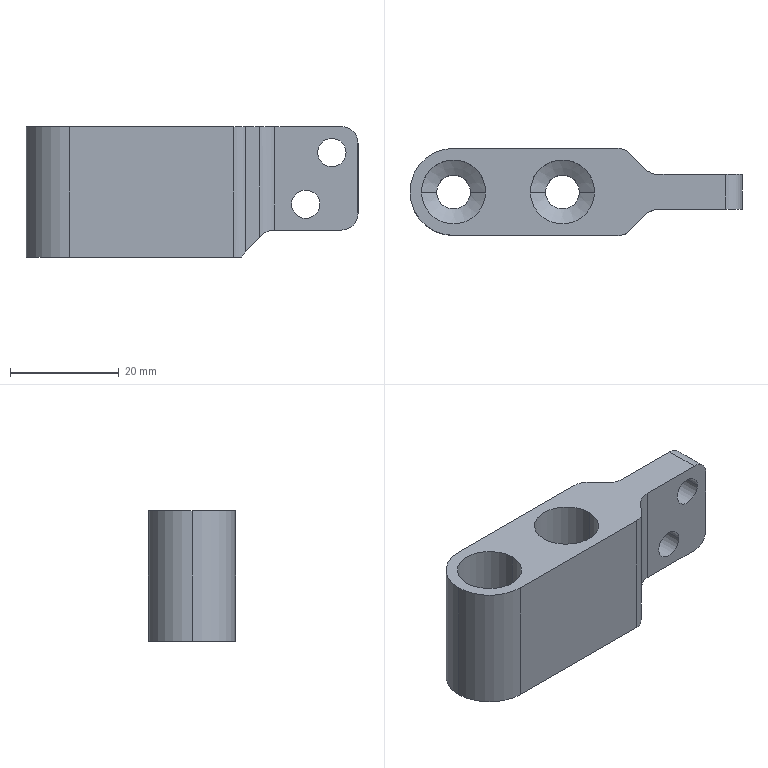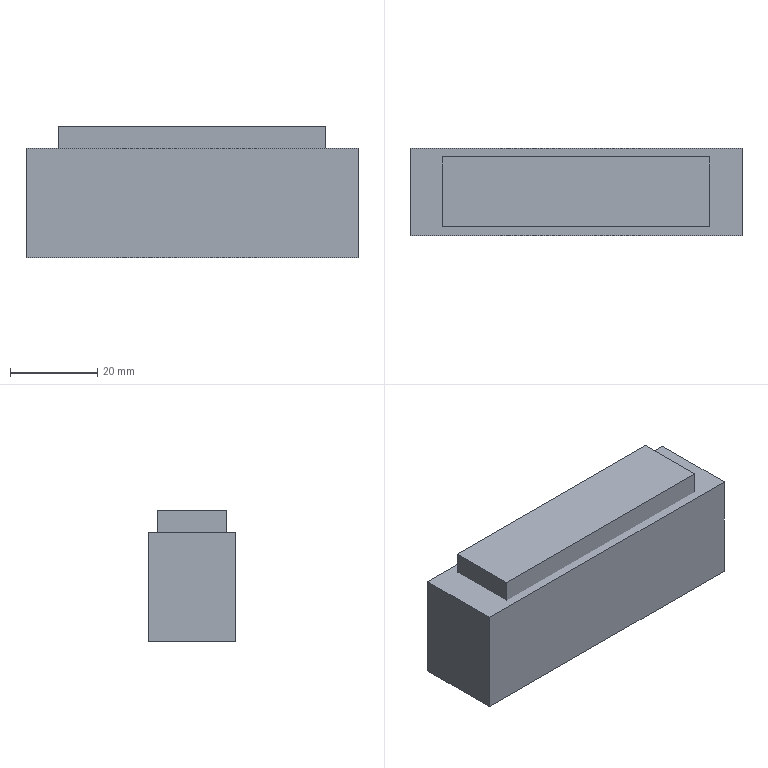CAM job | NX | 3+2 milling, drilling | part box 60.988 x 16 x 24 mm | stock box 75.988 x 20 x 30 mm
Tools:
number,name,description,diameter,corner_radius,flute_length,length,flutes
1,D63,Milling Tool-5 Parameters,63.0,0.0,50.0,75.0,2
7,D6A45,Milling Tool-5 Parameters,6.0,0.0,3.0,3.0,2
16,6.2ZT,Drilling Tool,6.2,0.0,35.0,50.0,2
12,11.8ZT,Drilling Tool,11.8,0.0,35.0,50.0,2
10,D10,Milling Tool-5 Parameters,10.0,0.0,50.0,75.0,2
11,D10JING,Milling Tool-5 Parameters,10.0,0.0,50.0,75.0,2
5,D6R0.5,Milling Tool-5 Parameters,6.0,0.5,50.0,75.0,2
15,5.2ZT,Drilling Tool,5.2,0.0,35.0,50.0,2
Operations:
program,operation,operation_type,tool,method,geometry_group,spindle_rpm,surface_speed,feed_per_tooth,feed_cut,feed_plunge,cut_length_mm,path_length_mm,cut_time_min,machine_time_min
1-30-18-73毛胚-G54-G55,FLOOR_WALL,VolumeBased25DMillingOperation,D63,METHOD,A,6500.0,1286.0,0.0962,1250.0,100.0,150.988,170.988,0.1208,0.1228
1-30-18-73毛胚-G54-G55,FLOOR_WALL_COPY_1,VolumeBased25DMillingOperation,D63,METHOD,AA,6500.0,1286.0,0.0962,1250.0,100.0,150.988,170.988,0.1208,0.1228
1-30-18-73毛胚-G54-G55,DRILLING_COPY_1,Operation,D6A45,METHOD,A,3000.0,56.0,0.0333,200.0,0.0,8.0,99.224,0.04,0.0491
1-30-18-73毛胚-G54-G55,DRILLING_COPY_1_COPY_2,Operation,D6A45,METHOD,AA,3000.0,56.0,0.0333,200.0,0.0,8.0,99.224,0.04,0.0491
1-30-18-73毛胚-G54-G55,DRILLING_COPY_1_COPY,Operation,6.2ZT,METHOD,A,2000.0,36.0,0.05,200.0,0.0,60.725,204.674,0.3036,0.318
1-30-18-73毛胚-G54-G55,DRILLING_COPY_1_COPY_COPY_2,Operation,6.2ZT,METHOD,AA,2000.0,36.0,0.05,200.0,0.0,60.725,204.674,0.3036,0.318
1-30-18-73毛胚-G54-G55,DRILLING_COPY_1_COPY_COPY,Operation,11.8ZT,METHOD,A,1500.0,55.0,0.0667,200.0,0.0,47.09,177.404,0.2355,0.2485
1-30-18-73毛胚-G54-G55,DRILLING_COPY_1_COPY_COPY_COPY,Operation,11.8ZT,METHOD,AA,1500.0,55.0,0.0667,200.0,0.0,47.09,177.404,0.2355,0.2485
1-30-18-73毛胚-G54-G55,ADAPTIVE_MILLING,CavityMilling,D10,METHOD,A,8000.0,251.0,0.2188,3500.0,1000.0,2896.63,3008.167,0.8319,0.843
1-30-18-73毛胚-G54-G55,ADAPTIVE_MILLING_COPY,CavityMilling,D10,METHOD,AA,8000.0,251.0,0.2188,3500.0,1000.0,2896.63,3008.167,0.8319,0.843
1-30-18-73毛胚-G54-G55,ZLEVEL_PROFILE_COPY_COPY_1,ZLevelMilling,D10JING,METHOD,A,8000.0,251.0,0.05,800.0,100.0,356.747,425.221,0.4459,0.4528
1-30-18-73毛胚-G54-G55,ZLEVEL_PROFILE_COPY_COPY_1_COPY,ZLevelMilling,D10JING,METHOD,AA,8000.0,251.0,0.05,800.0,100.0,356.747,425.221,0.4459,0.4528
1-30-18-73毛胚-G54-G55,ZLEVEL_PROFILE_COPY_1_COPY_1_COPY,ZLevelMilling,D6R0.5,METHOD,A,9500.0,89.0,0.1579,3000.0,1000.0,753.955,775.462,0.2537,0.2558
1-30-18-73毛胚-G54-G55,ZLEVEL_PROFILE_COPY_1_COPY_1_COPY_COPY,ZLevelMilling,D6R0.5,METHOD,A,9500.0,89.0,0.0868,1650.0,1000.0,478.198,834.903,0.3476,0.3833
1-30-18-73毛胚-G54-G55,ZLEVEL_PROFILE_COPY_1_COPY_1_COPY_COPY_2,ZLevelMilling,D6R0.5,METHOD,AA,9500.0,89.0,0.1579,3000.0,1000.0,753.955,775.462,0.2537,0.2558
1-30-18-73毛胚-G54-G55,ZLEVEL_PROFILE_COPY_1_COPY_1_COPY_COPY_COPY,ZLevelMilling,D6R0.5,METHOD,AA,9500.0,89.0,0.0868,1650.0,1000.0,478.198,834.903,0.3476,0.3833
1-30-18-73毛胚-G54-G55,ZLEVEL_PROFILE_COPY_1_COPY_COPY_COPY_COPY_2_COPY_COPY_1,ZLevelMilling,D6A45,METHOD,A,7000.0,131.0,0.0714,1000.0,1000.0,215.816,345.791,0.2158,0.2288
1-30-18-73毛胚-G54-G55,ZLEVEL_PROFILE_COPY_1_COPY_COPY_COPY_COPY_2_COPY_COPY_1_COPY_2,ZLevelMilling,D6A45,METHOD,AA,7000.0,131.0,0.0714,1000.0,1000.0,215.816,345.791,0.2158,0.2288
2-30-18-73毛胚-G54-G55,FLOOR_WALL_COPY,VolumeBased25DMillingOperation,D63,METHOD,B,6500.0,1286.0,0.0962,1250.0,100.0,815.927,1759.868,0.6527,0.7471
2-30-18-73毛胚-G54-G55,FLOOR_WALL_COPY_COPY,VolumeBased25DMillingOperation,D63,METHOD,B,6500.0,1286.0,0.0962,1250.0,100.0,407.3,1009.05,0.3258,0.386
2-30-18-73毛胚-G54-G55,FLOOR_WALL_COPY_COPY_1,VolumeBased25DMillingOperation,D63,METHOD,BB,6500.0,1286.0,0.0962,1250.0,100.0,815.927,1759.868,0.6527,0.7471
2-30-18-73毛胚-G54-G55,FLOOR_WALL_COPY_COPY_COPY,VolumeBased25DMillingOperation,D63,METHOD,BB,6500.0,1286.0,0.0962,1250.0,100.0,407.3,1009.05,0.3258,0.386
2-30-18-73毛胚-G54-G55,ZLEVEL_PROFILE_COPY_1_COPY_1_COPY_COPY_1,ZLevelMilling,D6R0.5,METHOD,B,9500.0,89.0,0.1579,3000.0,1000.0,1468.408,1529.483,0.4918,0.4979
2-30-18-73毛胚-G54-G55,ZLEVEL_PROFILE_COPY_1_COPY_1_COPY_COPY_1_COPY,ZLevelMilling,D6R0.5,METHOD,B,9500.0,89.0,0.1579,3000.0,1000.0,753.781,823.289,0.2536,0.2606
2-30-18-73毛胚-G54-G55,ZLEVEL_PROFILE_COPY_1_COPY_1_COPY_COPY_1_COPY_1,ZLevelMilling,D6R0.5,METHOD,BB,9500.0,89.0,0.1579,3000.0,1000.0,1468.408,1529.483,0.4918,0.4979
2-30-18-73毛胚-G54-G55,ZLEVEL_PROFILE_COPY_1_COPY_1_COPY_COPY_1_COPY_COPY,ZLevelMilling,D6R0.5,METHOD,BB,9500.0,89.0,0.1579,3000.0,1000.0,753.781,823.289,0.2536,0.2606
2-30-18-73毛胚-G54-G55,ZLEVEL_PROFILE_COPY_1_COPY_COPY_COPY_COPY_2_COPY_COPY_1_COPY,ZLevelMilling,D6A45,METHOD,B,7000.0,131.0,0.0714,1000.0,1000.0,139.991,364.977,0.14,0.1625
2-30-18-73毛胚-G54-G55,ZLEVEL_PROFILE_COPY_1_COPY_COPY_COPY_COPY_2_COPY_COPY_1_COPY_COPY,ZLevelMilling,D6A45,METHOD,B,7000.0,131.0,0.0714,1000.0,1000.0,42.107,200.377,0.0421,0.0579
2-30-18-73毛胚-G54-G55,ZLEVEL_PROFILE_COPY_1_COPY_COPY_COPY_COPY_2_COPY_COPY_1_COPY_COPY_1,ZLevelMilling,D6A45,METHOD,BB,7000.0,131.0,0.0714,1000.0,1000.0,139.991,364.977,0.14,0.1625
2-30-18-73毛胚-G54-G55,ZLEVEL_PROFILE_COPY_1_COPY_COPY_COPY_COPY_2_COPY_COPY_1_COPY_COPY_COPY,ZLevelMilling,D6A45,METHOD,BB,7000.0,131.0,0.0714,1000.0,1000.0,42.107,200.377,0.0421,0.0579
3-30-18-73毛胚-G54-G55,DRILLING_COPY_1_COPY_1,Operation,D6A45,METHOD,C,3000.0,56.0,0.0333,200.0,0.0,8.0,99.659,0.04,0.0492
3-30-18-73毛胚-G54-G55,DRILLING_COPY_1_COPY_1_COPY,Operation,D6A45,METHOD,CC,3000.0,56.0,0.0333,200.0,0.0,8.0,99.659,0.04,0.0492
3-30-18-73毛胚-G54-G55,DRILLING_COPY_1_COPY_COPY_1,Operation,5.2ZT,METHOD,C,2000.0,36.0,0.05,200.0,0.0,24.924,133.507,0.1246,0.1355
3-30-18-73毛胚-G54-G55,DRILLING_COPY_1_COPY_COPY_1_COPY,Operation,5.2ZT,METHOD,CC,2000.0,36.0,0.05,200.0,0.0,24.924,133.507,0.1246,0.1355
3-30-18-73毛胚-G54-G55,ZLEVEL_PROFILE_COPY_1_COPY_COPY_COPY_COPY_2_COPY_COPY_1_COPY_1,ZLevelMilling,D6A45,METHOD,C,7000.0,131.0,0.0714,1000.0,1000.0,23.044,178.908,0.023,0.0386
3-30-18-73毛胚-G54-G55,ZLEVEL_PROFILE_COPY_1_COPY_COPY_COPY_COPY_2_COPY_COPY_1_COPY_1_COPY,ZLevelMilling,D6A45,METHOD,CC,7000.0,131.0,0.0714,1000.0,1000.0,23.044,178.908,0.023,0.0386